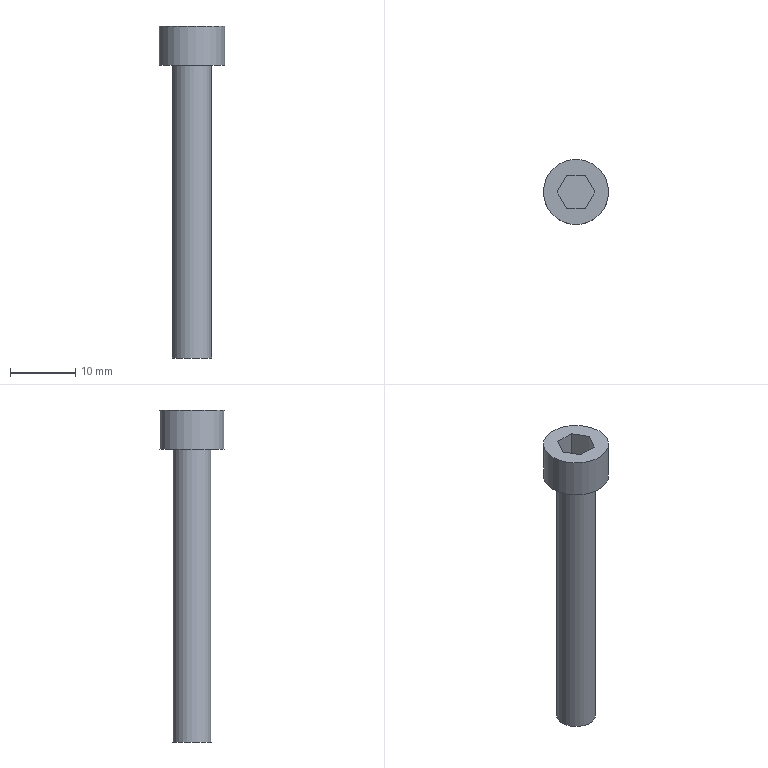Part | STEP file | 1 solid | 12 faces | box 10 x 10 x 51 mm | volume 1658 mm3 | plane 10 | cylinder 2 | commonest cylinder face diameters 6 x1 10 x1
STEP:
#1=CARTESIAN_POINT('',(0.,0.,0.));
#2=DIRECTION('',(0.,0.,1.));
#3=DIRECTION('',(1.,0.,0.));
#4=AXIS2_PLACEMENT_3D('',#1,#2,#3);
#5=CARTESIAN_POINT('',(1569.457,565.48,-58.253));
#6=VERTEX_POINT('',#5);
#7=CARTESIAN_POINT('',(1564.457,565.48,-58.253));
#8=DIRECTION('',(0.,0.,1.));
#9=DIRECTION('',(1.,0.,0.));
#10=AXIS2_PLACEMENT_3D('',#7,#8,#9);
#11=CIRCLE('',#10,5.);
#12=CARTESIAN_POINT('',(1569.457,565.48,-58.253));
#13=DIRECTION('',(0.,0.,-1.));
#14=DIRECTION('',(-1.,0.,0.));
#15=AXIS2_PLACEMENT_3D('',#12,#13,#14);
#16=PLANE('',#15);
#17=CARTESIAN_POINT('',(0.,0.));
#18=CARTESIAN_POINT('',(0.,8.66));
#19=CARTESIAN_POINT('',(7.5,4.33));
#20=CARTESIAN_POINT('',(15.,0.));
#21=CARTESIAN_POINT('',(7.5,-4.33));
#22=CARTESIAN_POINT('',(0.,-8.66));
#23=CARTESIAN_POINT('',(0.,0.));
#24=(BOUNDED_CURVE()B_SPLINE_CURVE(2,(#17,#18,#19,#20,#21,#22,#23),.UNSPECIFIED.,.T.,.F.)B_SPLINE_CURVE_WITH_KNOTS((1,2,2,2,2,1),(-2.094,0.,2.094,4.189,6.283,8.378),.UNSPECIFIED.)CURVE()GEOMETRIC_REPRESENTATION_ITEM()RATIONAL_B_SPLINE_CURVE((1.,0.5,1.,0.5,1.,0.5,1.))REPRESENTATION_ITEM(''));
#25=(GEOMETRIC_REPRESENTATION_CONTEXT(2)PARAMETRIC_REPRESENTATION_CONTEXT()REPRESENTATION_CONTEXT('',''));
#26=DEFINITIONAL_REPRESENTATION('',(#24),#25);
#27=PCURVE('',#16,#26);
#28=CARTESIAN_POINT('',(1564.457,565.48,-64.153));
#29=DIRECTION('',(0.,0.,1.));
#30=DIRECTION('',(1.,0.,0.));
#31=AXIS2_PLACEMENT_3D('',#28,#29,#30);
#32=CYLINDRICAL_SURFACE('',#31,5.);
#33=CARTESIAN_POINT('',(0.,5.9));
#34=DIRECTION('',(1.,0.));
#35=VECTOR('',#34,1.);
#36=LINE('',#33,#35);
#37=(GEOMETRIC_REPRESENTATION_CONTEXT(2)PARAMETRIC_REPRESENTATION_CONTEXT()REPRESENTATION_CONTEXT('',''));
#38=DEFINITIONAL_REPRESENTATION('',(#36),#37);
#39=PCURVE('',#32,#38);
#40=SURFACE_CURVE('',#11,(#27,#39),.PCURVE_S1.);
#41=EDGE_CURVE('',#6,#6,#40,.T.);
#42=ORIENTED_EDGE('',*,*,#41,.T.);
#43=EDGE_LOOP('',(#42));
#44=FACE_BOUND('',#43,.T.);
#45=CARTESIAN_POINT('',(1563.014,567.98,-58.253));
#46=VERTEX_POINT('',#45);
#47=CARTESIAN_POINT('',(1565.901,567.98,-58.253));
#48=VERTEX_POINT('',#47);
#49=CARTESIAN_POINT('',(1563.014,567.98,-58.253));
#50=DIRECTION('',(1.,0.,0.));
#51=VECTOR('',#50,1.);
#52=LINE('',#49,#51);
#53=CARTESIAN_POINT('',(6.443,2.5));
#54=DIRECTION('',(-1.,0.));
#55=VECTOR('',#54,1.);
#56=LINE('',#53,#55);
#57=(GEOMETRIC_REPRESENTATION_CONTEXT(2)PARAMETRIC_REPRESENTATION_CONTEXT()REPRESENTATION_CONTEXT('',''));
#58=DEFINITIONAL_REPRESENTATION('',(#56),#57);
#59=PCURVE('',#16,#58);
#60=CARTESIAN_POINT('',(1563.014,567.98,-62.213));
#61=DIRECTION('',(0.,-1.,0.));
#62=DIRECTION('',(1.,0.,0.));
#63=AXIS2_PLACEMENT_3D('',#60,#61,#62);
#64=PLANE('',#63);
#65=CARTESIAN_POINT('',(0.,3.96));
#66=DIRECTION('',(1.,0.));
#67=VECTOR('',#66,1.);
#68=LINE('',#65,#67);
#69=(GEOMETRIC_REPRESENTATION_CONTEXT(2)PARAMETRIC_REPRESENTATION_CONTEXT()REPRESENTATION_CONTEXT('',''));
#70=DEFINITIONAL_REPRESENTATION('',(#68),#69);
#71=PCURVE('',#64,#70);
#72=SURFACE_CURVE('',#52,(#59,#71),.PCURVE_S1.);
#73=EDGE_CURVE('',#46,#48,#72,.T.);
#74=ORIENTED_EDGE('',*,*,#73,.T.);
#75=CARTESIAN_POINT('',(1567.344,565.48,-58.253));
#76=VERTEX_POINT('',#75);
#77=CARTESIAN_POINT('',(1565.901,567.98,-58.253));
#78=DIRECTION('',(0.5,-0.866,0.));
#79=VECTOR('',#78,1.);
#80=LINE('',#77,#79);
#81=CARTESIAN_POINT('',(3.557,2.5));
#82=DIRECTION('',(-0.5,-0.866));
#83=VECTOR('',#82,1.);
#84=LINE('',#81,#83);
#85=(GEOMETRIC_REPRESENTATION_CONTEXT(2)PARAMETRIC_REPRESENTATION_CONTEXT()REPRESENTATION_CONTEXT('',''));
#86=DEFINITIONAL_REPRESENTATION('',(#84),#85);
#87=PCURVE('',#16,#86);
#88=CARTESIAN_POINT('',(1565.901,567.98,-62.213));
#89=DIRECTION('',(-0.866,-0.5,0.));
#90=DIRECTION('',(0.5,-0.866,0.));
#91=AXIS2_PLACEMENT_3D('',#88,#89,#90);
#92=PLANE('',#91);
#93=CARTESIAN_POINT('',(0.,3.96));
#94=DIRECTION('',(1.,0.));
#95=VECTOR('',#94,1.);
#96=LINE('',#93,#95);
#97=(GEOMETRIC_REPRESENTATION_CONTEXT(2)PARAMETRIC_REPRESENTATION_CONTEXT()REPRESENTATION_CONTEXT('',''));
#98=DEFINITIONAL_REPRESENTATION('',(#96),#97);
#99=PCURVE('',#92,#98);
#100=SURFACE_CURVE('',#80,(#87,#99),.PCURVE_S1.);
#101=EDGE_CURVE('',#48,#76,#100,.T.);
#102=ORIENTED_EDGE('',*,*,#101,.T.);
#103=CARTESIAN_POINT('',(1565.901,562.98,-58.253));
#104=VERTEX_POINT('',#103);
#105=CARTESIAN_POINT('',(1567.344,565.48,-58.253));
#106=DIRECTION('',(-0.5,-0.866,0.));
#107=VECTOR('',#106,1.);
#108=LINE('',#105,#107);
#109=CARTESIAN_POINT('',(2.113,0.));
#110=DIRECTION('',(0.5,-0.866));
#111=VECTOR('',#110,1.);
#112=LINE('',#109,#111);
#113=(GEOMETRIC_REPRESENTATION_CONTEXT(2)PARAMETRIC_REPRESENTATION_CONTEXT()REPRESENTATION_CONTEXT('',''));
#114=DEFINITIONAL_REPRESENTATION('',(#112),#113);
#115=PCURVE('',#16,#114);
#116=CARTESIAN_POINT('',(1567.344,565.48,-62.213));
#117=DIRECTION('',(-0.866,0.5,0.));
#118=DIRECTION('',(-0.5,-0.866,0.));
#119=AXIS2_PLACEMENT_3D('',#116,#117,#118);
#120=PLANE('',#119);
#121=CARTESIAN_POINT('',(0.,3.96));
#122=DIRECTION('',(1.,0.));
#123=VECTOR('',#122,1.);
#124=LINE('',#121,#123);
#125=(GEOMETRIC_REPRESENTATION_CONTEXT(2)PARAMETRIC_REPRESENTATION_CONTEXT()REPRESENTATION_CONTEXT('',''));
#126=DEFINITIONAL_REPRESENTATION('',(#124),#125);
#127=PCURVE('',#120,#126);
#128=SURFACE_CURVE('',#108,(#115,#127),.PCURVE_S1.);
#129=EDGE_CURVE('',#76,#104,#128,.T.);
#130=ORIENTED_EDGE('',*,*,#129,.T.);
#131=CARTESIAN_POINT('',(1563.014,562.98,-58.253));
#132=VERTEX_POINT('',#131);
#133=CARTESIAN_POINT('',(1565.901,562.98,-58.253));
#134=DIRECTION('',(-1.,0.,0.));
#135=VECTOR('',#134,1.);
#136=LINE('',#133,#135);
#137=CARTESIAN_POINT('',(3.557,-2.5));
#138=DIRECTION('',(1.,0.));
#139=VECTOR('',#138,1.);
#140=LINE('',#137,#139);
#141=(GEOMETRIC_REPRESENTATION_CONTEXT(2)PARAMETRIC_REPRESENTATION_CONTEXT()REPRESENTATION_CONTEXT('',''));
#142=DEFINITIONAL_REPRESENTATION('',(#140),#141);
#143=PCURVE('',#16,#142);
#144=CARTESIAN_POINT('',(1565.901,562.98,-62.213));
#145=DIRECTION('',(0.,1.,0.));
#146=DIRECTION('',(-1.,0.,0.));
#147=AXIS2_PLACEMENT_3D('',#144,#145,#146);
#148=PLANE('',#147);
#149=CARTESIAN_POINT('',(0.,3.96));
#150=DIRECTION('',(1.,0.));
#151=VECTOR('',#150,1.);
#152=LINE('',#149,#151);
#153=(GEOMETRIC_REPRESENTATION_CONTEXT(2)PARAMETRIC_REPRESENTATION_CONTEXT()REPRESENTATION_CONTEXT('',''));
#154=DEFINITIONAL_REPRESENTATION('',(#152),#153);
#155=PCURVE('',#148,#154);
#156=SURFACE_CURVE('',#136,(#143,#155),.PCURVE_S1.);
#157=EDGE_CURVE('',#104,#132,#156,.T.);
#158=ORIENTED_EDGE('',*,*,#157,.T.);
#159=CARTESIAN_POINT('',(1561.57,565.48,-58.253));
#160=VERTEX_POINT('',#159);
#161=CARTESIAN_POINT('',(1563.014,562.98,-58.253));
#162=DIRECTION('',(-0.5,0.866,0.));
#163=VECTOR('',#162,1.);
#164=LINE('',#161,#163);
#165=CARTESIAN_POINT('',(6.443,-2.5));
#166=DIRECTION('',(0.5,0.866));
#167=VECTOR('',#166,1.);
#168=LINE('',#165,#167);
#169=(GEOMETRIC_REPRESENTATION_CONTEXT(2)PARAMETRIC_REPRESENTATION_CONTEXT()REPRESENTATION_CONTEXT('',''));
#170=DEFINITIONAL_REPRESENTATION('',(#168),#169);
#171=PCURVE('',#16,#170);
#172=CARTESIAN_POINT('',(1563.014,562.98,-62.213));
#173=DIRECTION('',(0.866,0.5,0.));
#174=DIRECTION('',(-0.5,0.866,0.));
#175=AXIS2_PLACEMENT_3D('',#172,#173,#174);
#176=PLANE('',#175);
#177=CARTESIAN_POINT('',(0.,3.96));
#178=DIRECTION('',(1.,0.));
#179=VECTOR('',#178,1.);
#180=LINE('',#177,#179);
#181=(GEOMETRIC_REPRESENTATION_CONTEXT(2)PARAMETRIC_REPRESENTATION_CONTEXT()REPRESENTATION_CONTEXT('',''));
#182=DEFINITIONAL_REPRESENTATION('',(#180),#181);
#183=PCURVE('',#176,#182);
#184=SURFACE_CURVE('',#164,(#171,#183),.PCURVE_S1.);
#185=EDGE_CURVE('',#132,#160,#184,.T.);
#186=ORIENTED_EDGE('',*,*,#185,.T.);
#187=CARTESIAN_POINT('',(1561.57,565.48,-58.253));
#188=DIRECTION('',(0.5,0.866,0.));
#189=VECTOR('',#188,1.);
#190=LINE('',#187,#189);
#191=CARTESIAN_POINT('',(7.887,0.));
#192=DIRECTION('',(-0.5,0.866));
#193=VECTOR('',#192,1.);
#194=LINE('',#191,#193);
#195=(GEOMETRIC_REPRESENTATION_CONTEXT(2)PARAMETRIC_REPRESENTATION_CONTEXT()REPRESENTATION_CONTEXT('',''));
#196=DEFINITIONAL_REPRESENTATION('',(#194),#195);
#197=PCURVE('',#16,#196);
#198=CARTESIAN_POINT('',(1561.57,565.48,-62.213));
#199=DIRECTION('',(0.866,-0.5,0.));
#200=DIRECTION('',(0.5,0.866,0.));
#201=AXIS2_PLACEMENT_3D('',#198,#199,#200);
#202=PLANE('',#201);
#203=CARTESIAN_POINT('',(0.,3.96));
#204=DIRECTION('',(1.,0.));
#205=VECTOR('',#204,1.);
#206=LINE('',#203,#205);
#207=(GEOMETRIC_REPRESENTATION_CONTEXT(2)PARAMETRIC_REPRESENTATION_CONTEXT()REPRESENTATION_CONTEXT('',''));
#208=DEFINITIONAL_REPRESENTATION('',(#206),#207);
#209=PCURVE('',#202,#208);
#210=SURFACE_CURVE('',#190,(#197,#209),.PCURVE_S1.);
#211=EDGE_CURVE('',#160,#46,#210,.T.);
#212=ORIENTED_EDGE('',*,*,#211,.T.);
#213=EDGE_LOOP('',(#74,#102,#130,#158,#186,#212));
#214=FACE_BOUND('',#213,.T.);
#215=ADVANCED_FACE('',(#44,#214),#16,.F.);
#216=ORIENTED_EDGE('',*,*,#41,.F.);
#217=CARTESIAN_POINT('',(1569.457,565.48,-64.253));
#218=VERTEX_POINT('',#217);
#219=CARTESIAN_POINT('',(1569.457,565.48,-64.253));
#220=CARTESIAN_POINT('',(1569.457,565.48,-58.253));
#221=B_SPLINE_CURVE_WITH_KNOTS('',1,(#219,#220),.UNSPECIFIED.,.F.,.F.,(2,2),(-0.1,5.9),.PIECEWISE_BEZIER_KNOTS.);
#222=CARTESIAN_POINT('',(0.,0.));
#223=DIRECTION('',(0.,1.));
#224=VECTOR('',#223,1.);
#225=LINE('',#222,#224);
#226=(GEOMETRIC_REPRESENTATION_CONTEXT(2)PARAMETRIC_REPRESENTATION_CONTEXT()REPRESENTATION_CONTEXT('',''));
#227=DEFINITIONAL_REPRESENTATION('',(#225),#226);
#228=PCURVE('',#32,#227);
#229=CARTESIAN_POINT('',(6.283,0.));
#230=DIRECTION('',(0.,1.));
#231=VECTOR('',#230,1.);
#232=LINE('',#229,#231);
#233=(GEOMETRIC_REPRESENTATION_CONTEXT(2)PARAMETRIC_REPRESENTATION_CONTEXT()REPRESENTATION_CONTEXT('',''));
#234=DEFINITIONAL_REPRESENTATION('',(#232),#233);
#235=PCURVE('',#32,#234);
#236=SEAM_CURVE('',#221,(#228,#235),.PCURVE_S1.);
#237=EDGE_CURVE('',#218,#6,#236,.T.);
#238=ORIENTED_EDGE('',*,*,#237,.F.);
#239=CARTESIAN_POINT('',(1564.457,565.48,-64.253));
#240=DIRECTION('',(0.,0.,1.));
#241=DIRECTION('',(1.,0.,0.));
#242=AXIS2_PLACEMENT_3D('',#239,#240,#241);
#243=CIRCLE('',#242,5.);
#244=CARTESIAN_POINT('',(0.,-0.1));
#245=DIRECTION('',(1.,0.));
#246=VECTOR('',#245,1.);
#247=LINE('',#244,#246);
#248=(GEOMETRIC_REPRESENTATION_CONTEXT(2)PARAMETRIC_REPRESENTATION_CONTEXT()REPRESENTATION_CONTEXT('',''));
#249=DEFINITIONAL_REPRESENTATION('',(#247),#248);
#250=PCURVE('',#32,#249);
#251=CARTESIAN_POINT('',(1567.457,565.48,-64.253));
#252=DIRECTION('',(0.,0.,1.));
#253=DIRECTION('',(1.,0.,0.));
#254=AXIS2_PLACEMENT_3D('',#251,#252,#253);
#255=PLANE('',#254);
#256=CARTESIAN_POINT('',(-3.,0.));
#257=DIRECTION('',(1.,0.));
#258=AXIS2_PLACEMENT_2D('',#256,#257);
#259=CIRCLE('',#258,5.);
#260=(GEOMETRIC_REPRESENTATION_CONTEXT(2)PARAMETRIC_REPRESENTATION_CONTEXT()REPRESENTATION_CONTEXT('',''));
#261=DEFINITIONAL_REPRESENTATION('',(#259),#260);
#262=PCURVE('',#255,#261);
#263=SURFACE_CURVE('',#243,(#250,#262),.PCURVE_S1.);
#264=EDGE_CURVE('',#218,#218,#263,.T.);
#265=ORIENTED_EDGE('',*,*,#264,.T.);
#266=ORIENTED_EDGE('',*,*,#237,.T.);
#267=EDGE_LOOP('',(#216,#238,#265,#266));
#268=FACE_BOUND('',#267,.T.);
#269=ADVANCED_FACE('',(#268),#32,.T.);
#270=ORIENTED_EDGE('',*,*,#264,.F.);
#271=EDGE_LOOP('',(#270));
#272=FACE_BOUND('',#271,.T.);
#273=CARTESIAN_POINT('',(1567.457,565.48,-64.253));
#274=VERTEX_POINT('',#273);
#275=CARTESIAN_POINT('',(1564.457,565.48,-64.253));
#276=DIRECTION('',(0.,0.,1.));
#277=DIRECTION('',(1.,0.,0.));
#278=AXIS2_PLACEMENT_3D('',#275,#276,#277);
#279=CIRCLE('',#278,3.);
#280=CARTESIAN_POINT('',(-3.,0.));
#281=DIRECTION('',(1.,0.));
#282=AXIS2_PLACEMENT_2D('',#280,#281);
#283=CIRCLE('',#282,3.);
#284=(GEOMETRIC_REPRESENTATION_CONTEXT(2)PARAMETRIC_REPRESENTATION_CONTEXT()REPRESENTATION_CONTEXT('',''));
#285=DEFINITIONAL_REPRESENTATION('',(#283),#284);
#286=PCURVE('',#255,#285);
#287=CARTESIAN_POINT('',(1564.457,565.48,-64.153));
#288=DIRECTION('',(0.,0.,1.));
#289=DIRECTION('',(1.,0.,0.));
#290=AXIS2_PLACEMENT_3D('',#287,#288,#289);
#291=CYLINDRICAL_SURFACE('',#290,3.);
#292=CARTESIAN_POINT('',(0.,-0.1));
#293=DIRECTION('',(1.,0.));
#294=VECTOR('',#293,1.);
#295=LINE('',#292,#294);
#296=(GEOMETRIC_REPRESENTATION_CONTEXT(2)PARAMETRIC_REPRESENTATION_CONTEXT()REPRESENTATION_CONTEXT('',''));
#297=DEFINITIONAL_REPRESENTATION('',(#295),#296);
#298=PCURVE('',#291,#297);
#299=SURFACE_CURVE('',#279,(#286,#298),.PCURVE_S1.);
#300=EDGE_CURVE('',#274,#274,#299,.T.);
#301=ORIENTED_EDGE('',*,*,#300,.T.);
#302=EDGE_LOOP('',(#301));
#303=FACE_BOUND('',#302,.T.);
#304=ADVANCED_FACE('',(#272,#303),#255,.F.);
#305=ORIENTED_EDGE('',*,*,#300,.F.);
#306=CARTESIAN_POINT('',(1567.457,565.48,-109.253));
#307=VERTEX_POINT('',#306);
#308=CARTESIAN_POINT('',(1567.457,565.48,-109.253));
#309=CARTESIAN_POINT('',(1567.457,565.48,-64.253));
#310=B_SPLINE_CURVE_WITH_KNOTS('',1,(#308,#309),.UNSPECIFIED.,.F.,.F.,(2,2),(-45.1,-0.1),.PIECEWISE_BEZIER_KNOTS.);
#311=CARTESIAN_POINT('',(0.,0.));
#312=DIRECTION('',(0.,1.));
#313=VECTOR('',#312,1.);
#314=LINE('',#311,#313);
#315=(GEOMETRIC_REPRESENTATION_CONTEXT(2)PARAMETRIC_REPRESENTATION_CONTEXT()REPRESENTATION_CONTEXT('',''));
#316=DEFINITIONAL_REPRESENTATION('',(#314),#315);
#317=PCURVE('',#291,#316);
#318=CARTESIAN_POINT('',(6.283,0.));
#319=DIRECTION('',(0.,1.));
#320=VECTOR('',#319,1.);
#321=LINE('',#318,#320);
#322=(GEOMETRIC_REPRESENTATION_CONTEXT(2)PARAMETRIC_REPRESENTATION_CONTEXT()REPRESENTATION_CONTEXT('',''));
#323=DEFINITIONAL_REPRESENTATION('',(#321),#322);
#324=PCURVE('',#291,#323);
#325=SEAM_CURVE('',#310,(#317,#324),.PCURVE_S1.);
#326=EDGE_CURVE('',#307,#274,#325,.T.);
#327=ORIENTED_EDGE('',*,*,#326,.F.);
#328=CARTESIAN_POINT('',(1564.457,565.48,-109.253));
#329=DIRECTION('',(0.,0.,1.));
#330=DIRECTION('',(1.,0.,0.));
#331=AXIS2_PLACEMENT_3D('',#328,#329,#330);
#332=CIRCLE('',#331,3.);
#333=CARTESIAN_POINT('',(0.,-45.1));
#334=DIRECTION('',(1.,0.));
#335=VECTOR('',#334,1.);
#336=LINE('',#333,#335);
#337=(GEOMETRIC_REPRESENTATION_CONTEXT(2)PARAMETRIC_REPRESENTATION_CONTEXT()REPRESENTATION_CONTEXT('',''));
#338=DEFINITIONAL_REPRESENTATION('',(#336),#337);
#339=PCURVE('',#291,#338);
#340=CARTESIAN_POINT('',(1564.457,565.48,-109.253));
#341=DIRECTION('',(0.,0.,1.));
#342=DIRECTION('',(1.,0.,0.));
#343=AXIS2_PLACEMENT_3D('',#340,#341,#342);
#344=PLANE('',#343);
#345=CARTESIAN_POINT('',(0.,0.));
#346=DIRECTION('',(1.,0.));
#347=AXIS2_PLACEMENT_2D('',#345,#346);
#348=CIRCLE('',#347,3.);
#349=(GEOMETRIC_REPRESENTATION_CONTEXT(2)PARAMETRIC_REPRESENTATION_CONTEXT()REPRESENTATION_CONTEXT('',''));
#350=DEFINITIONAL_REPRESENTATION('',(#348),#349);
#351=PCURVE('',#344,#350);
#352=SURFACE_CURVE('',#332,(#339,#351),.PCURVE_S1.);
#353=EDGE_CURVE('',#307,#307,#352,.T.);
#354=ORIENTED_EDGE('',*,*,#353,.T.);
#355=ORIENTED_EDGE('',*,*,#326,.T.);
#356=EDGE_LOOP('',(#305,#327,#354,#355));
#357=FACE_BOUND('',#356,.T.);
#358=ADVANCED_FACE('',(#357),#291,.T.);
#359=ORIENTED_EDGE('',*,*,#353,.F.);
#360=EDGE_LOOP('',(#359));
#361=FACE_BOUND('',#360,.T.);
#362=ADVANCED_FACE('',(#361),#344,.F.);
#363=ORIENTED_EDGE('',*,*,#73,.F.);
#364=CARTESIAN_POINT('',(1563.014,567.98,-62.213));
#365=VERTEX_POINT('',#364);
#366=CARTESIAN_POINT('',(1563.014,567.98,-62.213));
#367=DIRECTION('',(0.,0.,-1.));
#368=VECTOR('',#367,1.);
#369=LINE('',#366,#368);
#370=CARTESIAN_POINT('',(0.,0.));
#371=DIRECTION('',(0.,-1.));
#372=VECTOR('',#371,1.);
#373=LINE('',#370,#372);
#374=(GEOMETRIC_REPRESENTATION_CONTEXT(2)PARAMETRIC_REPRESENTATION_CONTEXT()REPRESENTATION_CONTEXT('',''));
#375=DEFINITIONAL_REPRESENTATION('',(#373),#374);
#376=PCURVE('',#64,#375);
#377=CARTESIAN_POINT('',(2.887,0.));
#378=DIRECTION('',(0.,-1.));
#379=VECTOR('',#378,1.);
#380=LINE('',#377,#379);
#381=(GEOMETRIC_REPRESENTATION_CONTEXT(2)PARAMETRIC_REPRESENTATION_CONTEXT()REPRESENTATION_CONTEXT('',''));
#382=DEFINITIONAL_REPRESENTATION('',(#380),#381);
#383=PCURVE('',#202,#382);
#384=SURFACE_CURVE('',#369,(#376,#383),.PCURVE_S1.);
#385=EDGE_CURVE('',#46,#365,#384,.T.);
#386=ORIENTED_EDGE('',*,*,#385,.T.);
#387=CARTESIAN_POINT('',(1565.901,567.98,-62.213));
#388=VERTEX_POINT('',#387);
#389=CARTESIAN_POINT('',(1563.014,567.98,-62.213));
#390=DIRECTION('',(-1.,0.,0.));
#391=VECTOR('',#390,1.);
#392=LINE('',#389,#391);
#393=CARTESIAN_POINT('',(0.,0.));
#394=DIRECTION('',(-1.,0.));
#395=VECTOR('',#394,1.);
#396=LINE('',#393,#395);
#397=(GEOMETRIC_REPRESENTATION_CONTEXT(2)PARAMETRIC_REPRESENTATION_CONTEXT()REPRESENTATION_CONTEXT('',''));
#398=DEFINITIONAL_REPRESENTATION('',(#396),#397);
#399=PCURVE('',#64,#398);
#400=CARTESIAN_POINT('',(1564.457,565.48,-62.213));
#401=DIRECTION('',(0.,0.,-1.));
#402=DIRECTION('',(-1.,0.,0.));
#403=AXIS2_PLACEMENT_3D('',#400,#401,#402);
#404=PLANE('',#403);
#405=CARTESIAN_POINT('',(1.443,2.5));
#406=DIRECTION('',(1.,0.));
#407=VECTOR('',#406,1.);
#408=LINE('',#405,#407);
#409=(GEOMETRIC_REPRESENTATION_CONTEXT(2)PARAMETRIC_REPRESENTATION_CONTEXT()REPRESENTATION_CONTEXT('',''));
#410=DEFINITIONAL_REPRESENTATION('',(#408),#409);
#411=PCURVE('',#404,#410);
#412=SURFACE_CURVE('',#392,(#399,#411),.PCURVE_S1.);
#413=EDGE_CURVE('',#388,#365,#412,.T.);
#414=ORIENTED_EDGE('',*,*,#413,.F.);
#415=CARTESIAN_POINT('',(1565.901,567.98,-62.213));
#416=DIRECTION('',(0.,0.,-1.));
#417=VECTOR('',#416,1.);
#418=LINE('',#415,#417);
#419=CARTESIAN_POINT('',(2.887,0.));
#420=DIRECTION('',(0.,-1.));
#421=VECTOR('',#420,1.);
#422=LINE('',#419,#421);
#423=(GEOMETRIC_REPRESENTATION_CONTEXT(2)PARAMETRIC_REPRESENTATION_CONTEXT()REPRESENTATION_CONTEXT('',''));
#424=DEFINITIONAL_REPRESENTATION('',(#422),#423);
#425=PCURVE('',#64,#424);
#426=CARTESIAN_POINT('',(0.,0.));
#427=DIRECTION('',(0.,-1.));
#428=VECTOR('',#427,1.);
#429=LINE('',#426,#428);
#430=(GEOMETRIC_REPRESENTATION_CONTEXT(2)PARAMETRIC_REPRESENTATION_CONTEXT()REPRESENTATION_CONTEXT('',''));
#431=DEFINITIONAL_REPRESENTATION('',(#429),#430);
#432=PCURVE('',#92,#431);
#433=SURFACE_CURVE('',#418,(#425,#432),.PCURVE_S1.);
#434=EDGE_CURVE('',#48,#388,#433,.T.);
#435=ORIENTED_EDGE('',*,*,#434,.F.);
#436=EDGE_LOOP('',(#363,#386,#414,#435));
#437=FACE_BOUND('',#436,.T.);
#438=ADVANCED_FACE('',(#437),#64,.T.);
#439=ORIENTED_EDGE('',*,*,#101,.F.);
#440=ORIENTED_EDGE('',*,*,#434,.T.);
#441=CARTESIAN_POINT('',(1567.344,565.48,-62.213));
#442=VERTEX_POINT('',#441);
#443=CARTESIAN_POINT('',(1565.901,567.98,-62.213));
#444=DIRECTION('',(-0.5,0.866,0.));
#445=VECTOR('',#444,1.);
#446=LINE('',#443,#445);
#447=CARTESIAN_POINT('',(0.,0.));
#448=DIRECTION('',(-1.,0.));
#449=VECTOR('',#448,1.);
#450=LINE('',#447,#449);
#451=(GEOMETRIC_REPRESENTATION_CONTEXT(2)PARAMETRIC_REPRESENTATION_CONTEXT()REPRESENTATION_CONTEXT('',''));
#452=DEFINITIONAL_REPRESENTATION('',(#450),#451);
#453=PCURVE('',#92,#452);
#454=CARTESIAN_POINT('',(-1.443,2.5));
#455=DIRECTION('',(0.5,0.866));
#456=VECTOR('',#455,1.);
#457=LINE('',#454,#456);
#458=(GEOMETRIC_REPRESENTATION_CONTEXT(2)PARAMETRIC_REPRESENTATION_CONTEXT()REPRESENTATION_CONTEXT('',''));
#459=DEFINITIONAL_REPRESENTATION('',(#457),#458);
#460=PCURVE('',#404,#459);
#461=SURFACE_CURVE('',#446,(#453,#460),.PCURVE_S1.);
#462=EDGE_CURVE('',#442,#388,#461,.T.);
#463=ORIENTED_EDGE('',*,*,#462,.F.);
#464=CARTESIAN_POINT('',(1567.344,565.48,-62.213));
#465=DIRECTION('',(0.,0.,-1.));
#466=VECTOR('',#465,1.);
#467=LINE('',#464,#466);
#468=CARTESIAN_POINT('',(2.887,0.));
#469=DIRECTION('',(0.,-1.));
#470=VECTOR('',#469,1.);
#471=LINE('',#468,#470);
#472=(GEOMETRIC_REPRESENTATION_CONTEXT(2)PARAMETRIC_REPRESENTATION_CONTEXT()REPRESENTATION_CONTEXT('',''));
#473=DEFINITIONAL_REPRESENTATION('',(#471),#472);
#474=PCURVE('',#92,#473);
#475=CARTESIAN_POINT('',(0.,0.));
#476=DIRECTION('',(0.,-1.));
#477=VECTOR('',#476,1.);
#478=LINE('',#475,#477);
#479=(GEOMETRIC_REPRESENTATION_CONTEXT(2)PARAMETRIC_REPRESENTATION_CONTEXT()REPRESENTATION_CONTEXT('',''));
#480=DEFINITIONAL_REPRESENTATION('',(#478),#479);
#481=PCURVE('',#120,#480);
#482=SURFACE_CURVE('',#467,(#474,#481),.PCURVE_S1.);
#483=EDGE_CURVE('',#76,#442,#482,.T.);
#484=ORIENTED_EDGE('',*,*,#483,.F.);
#485=EDGE_LOOP('',(#439,#440,#463,#484));
#486=FACE_BOUND('',#485,.T.);
#487=ADVANCED_FACE('',(#486),#92,.T.);
#488=ORIENTED_EDGE('',*,*,#129,.F.);
#489=ORIENTED_EDGE('',*,*,#483,.T.);
#490=CARTESIAN_POINT('',(1565.901,562.98,-62.213));
#491=VERTEX_POINT('',#490);
#492=CARTESIAN_POINT('',(1567.344,565.48,-62.213));
#493=DIRECTION('',(0.5,0.866,0.));
#494=VECTOR('',#493,1.);
#495=LINE('',#492,#494);
#496=CARTESIAN_POINT('',(0.,0.));
#497=DIRECTION('',(-1.,0.));
#498=VECTOR('',#497,1.);
#499=LINE('',#496,#498);
#500=(GEOMETRIC_REPRESENTATION_CONTEXT(2)PARAMETRIC_REPRESENTATION_CONTEXT()REPRESENTATION_CONTEXT('',''));
#501=DEFINITIONAL_REPRESENTATION('',(#499),#500);
#502=PCURVE('',#120,#501);
#503=CARTESIAN_POINT('',(-2.887,0.));
#504=DIRECTION('',(-0.5,0.866));
#505=VECTOR('',#504,1.);
#506=LINE('',#503,#505);
#507=(GEOMETRIC_REPRESENTATION_CONTEXT(2)PARAMETRIC_REPRESENTATION_CONTEXT()REPRESENTATION_CONTEXT('',''));
#508=DEFINITIONAL_REPRESENTATION('',(#506),#507);
#509=PCURVE('',#404,#508);
#510=SURFACE_CURVE('',#495,(#502,#509),.PCURVE_S1.);
#511=EDGE_CURVE('',#491,#442,#510,.T.);
#512=ORIENTED_EDGE('',*,*,#511,.F.);
#513=CARTESIAN_POINT('',(1565.901,562.98,-62.213));
#514=DIRECTION('',(0.,0.,-1.));
#515=VECTOR('',#514,1.);
#516=LINE('',#513,#515);
#517=CARTESIAN_POINT('',(2.887,0.));
#518=DIRECTION('',(0.,-1.));
#519=VECTOR('',#518,1.);
#520=LINE('',#517,#519);
#521=(GEOMETRIC_REPRESENTATION_CONTEXT(2)PARAMETRIC_REPRESENTATION_CONTEXT()REPRESENTATION_CONTEXT('',''));
#522=DEFINITIONAL_REPRESENTATION('',(#520),#521);
#523=PCURVE('',#120,#522);
#524=CARTESIAN_POINT('',(0.,0.));
#525=DIRECTION('',(0.,-1.));
#526=VECTOR('',#525,1.);
#527=LINE('',#524,#526);
#528=(GEOMETRIC_REPRESENTATION_CONTEXT(2)PARAMETRIC_REPRESENTATION_CONTEXT()REPRESENTATION_CONTEXT('',''));
#529=DEFINITIONAL_REPRESENTATION('',(#527),#528);
#530=PCURVE('',#148,#529);
#531=SURFACE_CURVE('',#516,(#523,#530),.PCURVE_S1.);
#532=EDGE_CURVE('',#104,#491,#531,.T.);
#533=ORIENTED_EDGE('',*,*,#532,.F.);
#534=EDGE_LOOP('',(#488,#489,#512,#533));
#535=FACE_BOUND('',#534,.T.);
#536=ADVANCED_FACE('',(#535),#120,.T.);
#537=ORIENTED_EDGE('',*,*,#157,.F.);
#538=ORIENTED_EDGE('',*,*,#532,.T.);
#539=CARTESIAN_POINT('',(1563.014,562.98,-62.213));
#540=VERTEX_POINT('',#539);
#541=CARTESIAN_POINT('',(1565.901,562.98,-62.213));
#542=DIRECTION('',(1.,0.,0.));
#543=VECTOR('',#542,1.);
#544=LINE('',#541,#543);
#545=CARTESIAN_POINT('',(0.,0.));
#546=DIRECTION('',(-1.,0.));
#547=VECTOR('',#546,1.);
#548=LINE('',#545,#547);
#549=(GEOMETRIC_REPRESENTATION_CONTEXT(2)PARAMETRIC_REPRESENTATION_CONTEXT()REPRESENTATION_CONTEXT('',''));
#550=DEFINITIONAL_REPRESENTATION('',(#548),#549);
#551=PCURVE('',#148,#550);
#552=CARTESIAN_POINT('',(-1.443,-2.5));
#553=DIRECTION('',(-1.,0.));
#554=VECTOR('',#553,1.);
#555=LINE('',#552,#554);
#556=(GEOMETRIC_REPRESENTATION_CONTEXT(2)PARAMETRIC_REPRESENTATION_CONTEXT()REPRESENTATION_CONTEXT('',''));
#557=DEFINITIONAL_REPRESENTATION('',(#555),#556);
#558=PCURVE('',#404,#557);
#559=SURFACE_CURVE('',#544,(#551,#558),.PCURVE_S1.);
#560=EDGE_CURVE('',#540,#491,#559,.T.);
#561=ORIENTED_EDGE('',*,*,#560,.F.);
#562=CARTESIAN_POINT('',(1563.014,562.98,-62.213));
#563=DIRECTION('',(0.,0.,-1.));
#564=VECTOR('',#563,1.);
#565=LINE('',#562,#564);
#566=CARTESIAN_POINT('',(2.887,0.));
#567=DIRECTION('',(0.,-1.));
#568=VECTOR('',#567,1.);
#569=LINE('',#566,#568);
#570=(GEOMETRIC_REPRESENTATION_CONTEXT(2)PARAMETRIC_REPRESENTATION_CONTEXT()REPRESENTATION_CONTEXT('',''));
#571=DEFINITIONAL_REPRESENTATION('',(#569),#570);
#572=PCURVE('',#148,#571);
#573=CARTESIAN_POINT('',(0.,0.));
#574=DIRECTION('',(0.,-1.));
#575=VECTOR('',#574,1.);
#576=LINE('',#573,#575);
#577=(GEOMETRIC_REPRESENTATION_CONTEXT(2)PARAMETRIC_REPRESENTATION_CONTEXT()REPRESENTATION_CONTEXT('',''));
#578=DEFINITIONAL_REPRESENTATION('',(#576),#577);
#579=PCURVE('',#176,#578);
#580=SURFACE_CURVE('',#565,(#572,#579),.PCURVE_S1.);
#581=EDGE_CURVE('',#132,#540,#580,.T.);
#582=ORIENTED_EDGE('',*,*,#581,.F.);
#583=EDGE_LOOP('',(#537,#538,#561,#582));
#584=FACE_BOUND('',#583,.T.);
#585=ADVANCED_FACE('',(#584),#148,.T.);
#586=ORIENTED_EDGE('',*,*,#185,.F.);
#587=ORIENTED_EDGE('',*,*,#581,.T.);
#588=CARTESIAN_POINT('',(1561.57,565.48,-62.213));
#589=VERTEX_POINT('',#588);
#590=CARTESIAN_POINT('',(1563.014,562.98,-62.213));
#591=DIRECTION('',(0.5,-0.866,0.));
#592=VECTOR('',#591,1.);
#593=LINE('',#590,#592);
#594=CARTESIAN_POINT('',(0.,0.));
#595=DIRECTION('',(-1.,0.));
#596=VECTOR('',#595,1.);
#597=LINE('',#594,#596);
#598=(GEOMETRIC_REPRESENTATION_CONTEXT(2)PARAMETRIC_REPRESENTATION_CONTEXT()REPRESENTATION_CONTEXT('',''));
#599=DEFINITIONAL_REPRESENTATION('',(#597),#598);
#600=PCURVE('',#176,#599);
#601=CARTESIAN_POINT('',(1.443,-2.5));
#602=DIRECTION('',(-0.5,-0.866));
#603=VECTOR('',#602,1.);
#604=LINE('',#601,#603);
#605=(GEOMETRIC_REPRESENTATION_CONTEXT(2)PARAMETRIC_REPRESENTATION_CONTEXT()REPRESENTATION_CONTEXT('',''));
#606=DEFINITIONAL_REPRESENTATION('',(#604),#605);
#607=PCURVE('',#404,#606);
#608=SURFACE_CURVE('',#593,(#600,#607),.PCURVE_S1.);
#609=EDGE_CURVE('',#589,#540,#608,.T.);
#610=ORIENTED_EDGE('',*,*,#609,.F.);
#611=CARTESIAN_POINT('',(1561.57,565.48,-62.213));
#612=DIRECTION('',(0.,0.,-1.));
#613=VECTOR('',#612,1.);
#614=LINE('',#611,#613);
#615=CARTESIAN_POINT('',(2.887,0.));
#616=DIRECTION('',(0.,-1.));
#617=VECTOR('',#616,1.);
#618=LINE('',#615,#617);
#619=(GEOMETRIC_REPRESENTATION_CONTEXT(2)PARAMETRIC_REPRESENTATION_CONTEXT()REPRESENTATION_CONTEXT('',''));
#620=DEFINITIONAL_REPRESENTATION('',(#618),#619);
#621=PCURVE('',#176,#620);
#622=CARTESIAN_POINT('',(0.,0.));
#623=DIRECTION('',(0.,-1.));
#624=VECTOR('',#623,1.);
#625=LINE('',#622,#624);
#626=(GEOMETRIC_REPRESENTATION_CONTEXT(2)PARAMETRIC_REPRESENTATION_CONTEXT()REPRESENTATION_CONTEXT('',''));
#627=DEFINITIONAL_REPRESENTATION('',(#625),#626);
#628=PCURVE('',#202,#627);
#629=SURFACE_CURVE('',#614,(#621,#628),.PCURVE_S1.);
#630=EDGE_CURVE('',#160,#589,#629,.T.);
#631=ORIENTED_EDGE('',*,*,#630,.F.);
#632=EDGE_LOOP('',(#586,#587,#610,#631));
#633=FACE_BOUND('',#632,.T.);
#634=ADVANCED_FACE('',(#633),#176,.T.);
#635=ORIENTED_EDGE('',*,*,#211,.F.);
#636=ORIENTED_EDGE('',*,*,#630,.T.);
#637=CARTESIAN_POINT('',(1561.57,565.48,-62.213));
#638=DIRECTION('',(-0.5,-0.866,0.));
#639=VECTOR('',#638,1.);
#640=LINE('',#637,#639);
#641=CARTESIAN_POINT('',(0.,0.));
#642=DIRECTION('',(-1.,0.));
#643=VECTOR('',#642,1.);
#644=LINE('',#641,#643);
#645=(GEOMETRIC_REPRESENTATION_CONTEXT(2)PARAMETRIC_REPRESENTATION_CONTEXT()REPRESENTATION_CONTEXT('',''));
#646=DEFINITIONAL_REPRESENTATION('',(#644),#645);
#647=PCURVE('',#202,#646);
#648=CARTESIAN_POINT('',(2.887,0.));
#649=DIRECTION('',(0.5,-0.866));
#650=VECTOR('',#649,1.);
#651=LINE('',#648,#650);
#652=(GEOMETRIC_REPRESENTATION_CONTEXT(2)PARAMETRIC_REPRESENTATION_CONTEXT()REPRESENTATION_CONTEXT('',''));
#653=DEFINITIONAL_REPRESENTATION('',(#651),#652);
#654=PCURVE('',#404,#653);
#655=SURFACE_CURVE('',#640,(#647,#654),.PCURVE_S1.);
#656=EDGE_CURVE('',#365,#589,#655,.T.);
#657=ORIENTED_EDGE('',*,*,#656,.F.);
#658=ORIENTED_EDGE('',*,*,#385,.F.);
#659=EDGE_LOOP('',(#635,#636,#657,#658));
#660=FACE_BOUND('',#659,.T.);
#661=ADVANCED_FACE('',(#660),#202,.T.);
#662=ORIENTED_EDGE('',*,*,#413,.T.);
#663=ORIENTED_EDGE('',*,*,#656,.T.);
#664=ORIENTED_EDGE('',*,*,#609,.T.);
#665=ORIENTED_EDGE('',*,*,#560,.T.);
#666=ORIENTED_EDGE('',*,*,#511,.T.);
#667=ORIENTED_EDGE('',*,*,#462,.T.);
#668=EDGE_LOOP('',(#662,#663,#664,#665,#666,#667));
#669=FACE_BOUND('',#668,.T.);
#670=ADVANCED_FACE('',(#669),#404,.F.);
#671=CLOSED_SHELL('',(#215,#269,#304,#358,#362,#438,#487,#536,#585,#634,#661,#670));
#672=MANIFOLD_SOLID_BREP('',#671);
#673=(LENGTH_UNIT()NAMED_UNIT(*)SI_UNIT(.MILLI.,.METRE.));
#674=UNCERTAINTY_MEASURE_WITH_UNIT(LENGTH_MEASURE(0.000002),#673,'','');
#675=(NAMED_UNIT(*)PLANE_ANGLE_UNIT()SI_UNIT($,.RADIAN.));
#676=(NAMED_UNIT(*)SI_UNIT($,.STERADIAN.)SOLID_ANGLE_UNIT());
#677=(GEOMETRIC_REPRESENTATION_CONTEXT(3)GLOBAL_UNCERTAINTY_ASSIGNED_CONTEXT((#674))GLOBAL_UNIT_ASSIGNED_CONTEXT((#673,#675,#676))REPRESENTATION_CONTEXT('',''));
#678=ADVANCED_BREP_SHAPE_REPRESENTATION('',(#4,#672),#677);